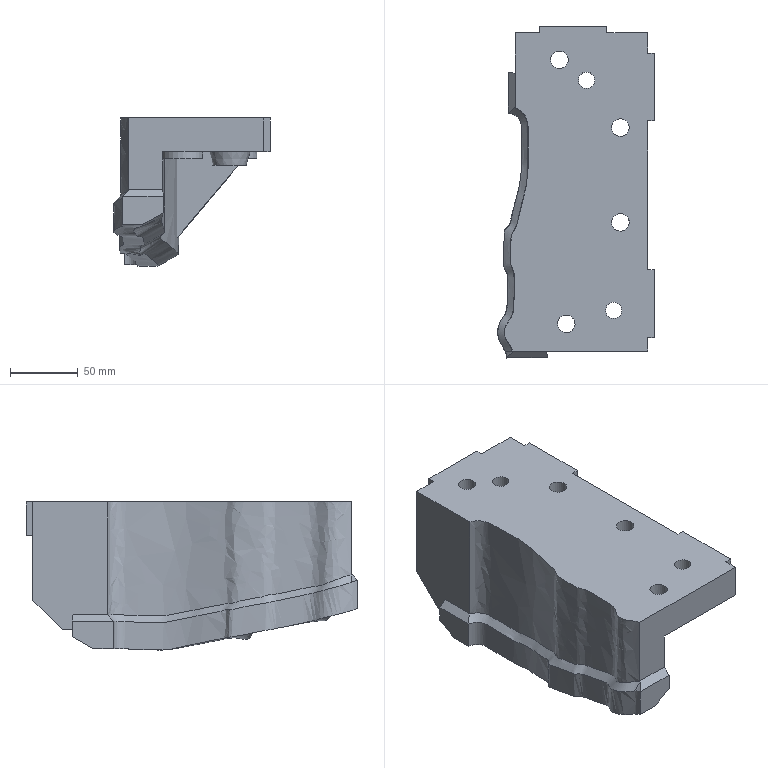Part | NX | features solid 2 | 1 solid | 58 faces | box 115.609 x 245 x 109.365 mm | volume 1066352 mm3 | plane 34 | cylinder 13 | spline 9 | cone 2 | commonest cylinder face diameters 13 x6 30 x5 12 x2